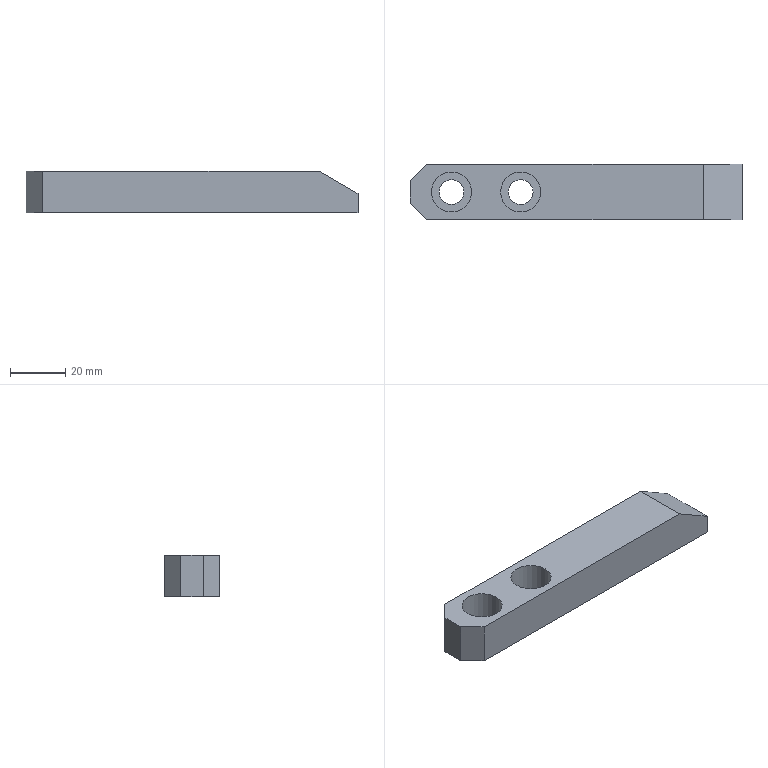Part | STEP file | lll_id830_x_t | 1 solid | 15 faces | box 120 x 20 x 15 mm | volume 30182 mm3 | plane 11 | cylinder 4 | commonest cylinder face diameters 9.009 x2 14.508 x2
STEP:
#1=CARTESIAN_POINT('',(3719.989,-179.337,0.));
#2=VERTEX_POINT('',#1);
#3=CARTESIAN_POINT('',(3727.243,-179.337,0.));
#4=DIRECTION('',(0.,0.,1.));
#5=DIRECTION('',(-1.,0.,0.));
#6=AXIS2_PLACEMENT_3D('',#3,#4,#5);
#7=CIRCLE('',#6,7.254);
#8=EDGE_CURVE('',#2,#2,#7,.T.);
#9=ORIENTED_EDGE('',*,*,#8,.F.);
#10=EDGE_LOOP('',(#9));
#11=FACE_BOUND('',#10,.T.);
#12=CARTESIAN_POINT('',(3694.989,-179.337,0.));
#13=VERTEX_POINT('',#12);
#14=CARTESIAN_POINT('',(3702.243,-179.337,0.));
#15=DIRECTION('',(0.,0.,1.));
#16=DIRECTION('',(-1.,0.,0.));
#17=AXIS2_PLACEMENT_3D('',#14,#15,#16);
#18=CIRCLE('',#17,7.254);
#19=EDGE_CURVE('',#13,#13,#18,.T.);
#20=ORIENTED_EDGE('',*,*,#19,.F.);
#21=EDGE_LOOP('',(#20));
#22=FACE_BOUND('',#21,.T.);
#23=CARTESIAN_POINT('',(3793.243,-169.337,0.));
#24=VERTEX_POINT('',#23);
#25=CARTESIAN_POINT('',(3693.243,-169.337,0.));
#26=VERTEX_POINT('',#25);
#27=CARTESIAN_POINT('',(3807.243,-169.337,0.));
#28=DIRECTION('',(-1.,0.,0.));
#29=VECTOR('',#28,1.);
#30=LINE('',#27,#29);
#31=EDGE_CURVE('',#24,#26,#30,.T.);
#32=ORIENTED_EDGE('',*,*,#31,.T.);
#33=CARTESIAN_POINT('',(3687.243,-175.337,0.));
#34=VERTEX_POINT('',#33);
#35=CARTESIAN_POINT('',(3687.243,-175.337,0.));
#36=DIRECTION('',(0.7071,0.7071,0.));
#37=VECTOR('',#36,1.);
#38=LINE('',#35,#37);
#39=EDGE_CURVE('',#34,#26,#38,.T.);
#40=ORIENTED_EDGE('',*,*,#39,.F.);
#41=CARTESIAN_POINT('',(3687.243,-183.337,0.));
#42=VERTEX_POINT('',#41);
#43=CARTESIAN_POINT('',(3687.243,-189.337,0.));
#44=DIRECTION('',(0.,1.,0.));
#45=VECTOR('',#44,1.);
#46=LINE('',#43,#45);
#47=EDGE_CURVE('',#42,#34,#46,.T.);
#48=ORIENTED_EDGE('',*,*,#47,.F.);
#49=CARTESIAN_POINT('',(3693.243,-189.337,0.));
#50=VERTEX_POINT('',#49);
#51=CARTESIAN_POINT('',(3693.243,-189.337,0.));
#52=DIRECTION('',(-0.7071,0.7071,0.));
#53=VECTOR('',#52,1.);
#54=LINE('',#51,#53);
#55=EDGE_CURVE('',#50,#42,#54,.T.);
#56=ORIENTED_EDGE('',*,*,#55,.F.);
#57=CARTESIAN_POINT('',(3793.243,-189.337,0.));
#58=VERTEX_POINT('',#57);
#59=CARTESIAN_POINT('',(3807.243,-189.337,0.));
#60=DIRECTION('',(-1.,0.,0.));
#61=VECTOR('',#60,1.);
#62=LINE('',#59,#61);
#63=EDGE_CURVE('',#58,#50,#62,.T.);
#64=ORIENTED_EDGE('',*,*,#63,.F.);
#65=CARTESIAN_POINT('',(3793.243,10.,0.));
#66=DIRECTION('',(0.,-1.,0.));
#67=VECTOR('',#66,1.);
#68=LINE('',#65,#67);
#69=EDGE_CURVE('',#24,#58,#68,.T.);
#70=ORIENTED_EDGE('',*,*,#69,.F.);
#71=EDGE_LOOP('',(#32,#40,#48,#56,#64,#70));
#72=FACE_BOUND('',#71,.T.);
#73=CARTESIAN_POINT('',(3807.243,-189.337,0.));
#74=DIRECTION('',(0.,0.,-1.));
#75=DIRECTION('',(1.,0.,0.));
#76=AXIS2_PLACEMENT_3D('',#73,#74,#75);
#77=PLANE('',#76);
#78=ADVANCED_FACE('',(#11,#22,#72),#77,.F.);
#79=CARTESIAN_POINT('',(3807.243,-169.337,-15.));
#80=VERTEX_POINT('',#79);
#81=CARTESIAN_POINT('',(3807.243,-169.337,-8.083));
#82=VERTEX_POINT('',#81);
#83=CARTESIAN_POINT('',(3807.243,-169.337,0.));
#84=DIRECTION('',(0.,0.,1.));
#85=VECTOR('',#84,1.);
#86=LINE('',#83,#85);
#87=EDGE_CURVE('',#80,#82,#86,.T.);
#88=ORIENTED_EDGE('',*,*,#87,.F.);
#89=CARTESIAN_POINT('',(3693.243,-169.337,-15.));
#90=VERTEX_POINT('',#89);
#91=CARTESIAN_POINT('',(3757.243,-169.337,-15.));
#92=DIRECTION('',(1.,0.,0.));
#93=VECTOR('',#92,1.);
#94=LINE('',#91,#93);
#95=EDGE_CURVE('',#90,#80,#94,.T.);
#96=ORIENTED_EDGE('',*,*,#95,.F.);
#97=CARTESIAN_POINT('',(3693.243,-169.337,-17.5));
#98=DIRECTION('',(0.,0.,-1.));
#99=VECTOR('',#98,1.);
#100=LINE('',#97,#99);
#101=EDGE_CURVE('',#26,#90,#100,.T.);
#102=ORIENTED_EDGE('',*,*,#101,.F.);
#103=ORIENTED_EDGE('',*,*,#31,.F.);
#104=CARTESIAN_POINT('',(3806.743,-169.337,-7.794));
#105=DIRECTION('',(-0.866,0.,0.5));
#106=VECTOR('',#105,1.);
#107=LINE('',#104,#106);
#108=EDGE_CURVE('',#82,#24,#107,.T.);
#109=ORIENTED_EDGE('',*,*,#108,.F.);
#110=EDGE_LOOP('',(#88,#96,#102,#103,#109));
#111=FACE_OUTER_BOUND('',#110,.T.);
#112=CARTESIAN_POINT('',(3757.243,-169.337,-17.5));
#113=DIRECTION('',(0.,-1.,0.));
#114=DIRECTION('',(0.,0.,-1.));
#115=AXIS2_PLACEMENT_3D('',#112,#113,#114);
#116=PLANE('',#115);
#117=ADVANCED_FACE('',(#111),#116,.F.);
#118=CARTESIAN_POINT('',(3687.243,-175.337,-15.));
#119=VERTEX_POINT('',#118);
#120=CARTESIAN_POINT('',(3687.243,-183.337,-15.));
#121=VERTEX_POINT('',#120);
#122=CARTESIAN_POINT('',(3687.243,10.,-15.));
#123=DIRECTION('',(0.,-1.,0.));
#124=VECTOR('',#123,1.);
#125=LINE('',#122,#124);
#126=EDGE_CURVE('',#119,#121,#125,.T.);
#127=ORIENTED_EDGE('',*,*,#126,.T.);
#128=CARTESIAN_POINT('',(3687.243,-183.337,0.));
#129=DIRECTION('',(0.,0.,-1.));
#130=VECTOR('',#129,1.);
#131=LINE('',#128,#130);
#132=EDGE_CURVE('',#42,#121,#131,.T.);
#133=ORIENTED_EDGE('',*,*,#132,.F.);
#134=ORIENTED_EDGE('',*,*,#47,.T.);
#135=CARTESIAN_POINT('',(3687.243,-175.337,0.));
#136=DIRECTION('',(0.,0.,1.));
#137=VECTOR('',#136,1.);
#138=LINE('',#135,#137);
#139=EDGE_CURVE('',#119,#34,#138,.T.);
#140=ORIENTED_EDGE('',*,*,#139,.F.);
#141=EDGE_LOOP('',(#127,#133,#134,#140));
#142=FACE_OUTER_BOUND('',#141,.T.);
#143=CARTESIAN_POINT('',(3687.243,10.,0.));
#144=DIRECTION('',(1.,0.,0.));
#145=DIRECTION('',(0.,0.,1.));
#146=AXIS2_PLACEMENT_3D('',#143,#144,#145);
#147=PLANE('',#146);
#148=ADVANCED_FACE('',(#142),#147,.F.);
#149=CARTESIAN_POINT('',(3807.243,-189.337,-15.));
#150=VERTEX_POINT('',#149);
#151=CARTESIAN_POINT('',(3807.243,-189.337,-8.083));
#152=VERTEX_POINT('',#151);
#153=CARTESIAN_POINT('',(3807.243,-189.337,-35.));
#154=DIRECTION('',(0.,0.,1.));
#155=VECTOR('',#154,1.);
#156=LINE('',#153,#155);
#157=EDGE_CURVE('',#150,#152,#156,.T.);
#158=ORIENTED_EDGE('',*,*,#157,.F.);
#159=CARTESIAN_POINT('',(3807.243,10.,-15.));
#160=DIRECTION('',(0.,1.,0.));
#161=VECTOR('',#160,1.);
#162=LINE('',#159,#161);
#163=EDGE_CURVE('',#150,#80,#162,.T.);
#164=ORIENTED_EDGE('',*,*,#163,.T.);
#165=ORIENTED_EDGE('',*,*,#87,.T.);
#166=CARTESIAN_POINT('',(3807.243,10.,-8.083));
#167=DIRECTION('',(0.,1.,0.));
#168=VECTOR('',#167,1.);
#169=LINE('',#166,#168);
#170=EDGE_CURVE('',#152,#82,#169,.T.);
#171=ORIENTED_EDGE('',*,*,#170,.F.);
#172=EDGE_LOOP('',(#158,#164,#165,#171));
#173=FACE_OUTER_BOUND('',#172,.T.);
#174=CARTESIAN_POINT('',(3807.243,10.,0.));
#175=DIRECTION('',(1.,0.,0.));
#176=DIRECTION('',(0.,0.,1.));
#177=AXIS2_PLACEMENT_3D('',#174,#175,#176);
#178=PLANE('',#177);
#179=ADVANCED_FACE('',(#173),#178,.T.);
#180=ORIENTED_EDGE('',*,*,#63,.T.);
#181=CARTESIAN_POINT('',(3693.243,-189.337,-15.));
#182=VERTEX_POINT('',#181);
#183=CARTESIAN_POINT('',(3693.243,-189.337,-35.));
#184=DIRECTION('',(0.,0.,1.));
#185=VECTOR('',#184,1.);
#186=LINE('',#183,#185);
#187=EDGE_CURVE('',#182,#50,#186,.T.);
#188=ORIENTED_EDGE('',*,*,#187,.F.);
#189=CARTESIAN_POINT('',(3807.243,-189.337,-15.));
#190=DIRECTION('',(1.,0.,0.));
#191=VECTOR('',#190,1.);
#192=LINE('',#189,#191);
#193=EDGE_CURVE('',#182,#150,#192,.T.);
#194=ORIENTED_EDGE('',*,*,#193,.T.);
#195=ORIENTED_EDGE('',*,*,#157,.T.);
#196=CARTESIAN_POINT('',(3806.743,-189.337,-7.794));
#197=DIRECTION('',(0.866,0.,-0.5));
#198=VECTOR('',#197,1.);
#199=LINE('',#196,#198);
#200=EDGE_CURVE('',#58,#152,#199,.T.);
#201=ORIENTED_EDGE('',*,*,#200,.F.);
#202=EDGE_LOOP('',(#180,#188,#194,#195,#201));
#203=FACE_OUTER_BOUND('',#202,.T.);
#204=CARTESIAN_POINT('',(3807.243,-189.337,-35.));
#205=DIRECTION('',(0.,1.,0.));
#206=DIRECTION('',(0.,0.,1.));
#207=AXIS2_PLACEMENT_3D('',#204,#205,#206);
#208=PLANE('',#207);
#209=ADVANCED_FACE('',(#203),#208,.F.);
#210=CARTESIAN_POINT('',(3722.739,-179.337,-15.));
#211=VERTEX_POINT('',#210);
#212=CARTESIAN_POINT('',(3727.243,-179.337,-15.));
#213=DIRECTION('',(0.,0.,-1.));
#214=DIRECTION('',(-1.,0.,0.));
#215=AXIS2_PLACEMENT_3D('',#212,#213,#214);
#216=CIRCLE('',#215,4.505);
#217=EDGE_CURVE('',#211,#211,#216,.T.);
#218=ORIENTED_EDGE('',*,*,#217,.F.);
#219=EDGE_LOOP('',(#218));
#220=FACE_BOUND('',#219,.T.);
#221=CARTESIAN_POINT('',(3697.739,-179.337,-15.));
#222=VERTEX_POINT('',#221);
#223=CARTESIAN_POINT('',(3702.243,-179.337,-15.));
#224=DIRECTION('',(0.,0.,-1.));
#225=DIRECTION('',(-1.,0.,0.));
#226=AXIS2_PLACEMENT_3D('',#223,#224,#225);
#227=CIRCLE('',#226,4.505);
#228=EDGE_CURVE('',#222,#222,#227,.T.);
#229=ORIENTED_EDGE('',*,*,#228,.F.);
#230=EDGE_LOOP('',(#229));
#231=FACE_BOUND('',#230,.T.);
#232=ORIENTED_EDGE('',*,*,#95,.T.);
#233=ORIENTED_EDGE('',*,*,#163,.F.);
#234=ORIENTED_EDGE('',*,*,#193,.F.);
#235=CARTESIAN_POINT('',(3693.243,-189.337,-15.));
#236=DIRECTION('',(0.7071,-0.7071,0.));
#237=VECTOR('',#236,1.);
#238=LINE('',#235,#237);
#239=EDGE_CURVE('',#121,#182,#238,.T.);
#240=ORIENTED_EDGE('',*,*,#239,.F.);
#241=ORIENTED_EDGE('',*,*,#126,.F.);
#242=CARTESIAN_POINT('',(3687.243,-175.337,-15.));
#243=DIRECTION('',(-0.7071,-0.7071,0.));
#244=VECTOR('',#243,1.);
#245=LINE('',#242,#244);
#246=EDGE_CURVE('',#90,#119,#245,.T.);
#247=ORIENTED_EDGE('',*,*,#246,.F.);
#248=EDGE_LOOP('',(#232,#233,#234,#240,#241,#247));
#249=FACE_BOUND('',#248,.T.);
#250=CARTESIAN_POINT('',(3757.243,-179.337,-15.));
#251=DIRECTION('',(0.,0.,1.));
#252=DIRECTION('',(-1.,0.,0.));
#253=AXIS2_PLACEMENT_3D('',#250,#251,#252);
#254=PLANE('',#253);
#255=ADVANCED_FACE('',(#220,#231,#249),#254,.F.);
#256=CARTESIAN_POINT('',(3697.739,-179.337,-11.));
#257=VERTEX_POINT('',#256);
#258=CARTESIAN_POINT('',(3702.243,-179.337,-11.));
#259=DIRECTION('',(0.,0.,1.));
#260=DIRECTION('',(-1.,0.,0.));
#261=AXIS2_PLACEMENT_3D('',#258,#259,#260);
#262=CIRCLE('',#261,4.505);
#263=EDGE_CURVE('',#257,#257,#262,.T.);
#264=ORIENTED_EDGE('',*,*,#263,.T.);
#265=EDGE_LOOP('',(#264));
#266=FACE_BOUND('',#265,.T.);
#267=ORIENTED_EDGE('',*,*,#228,.T.);
#268=EDGE_LOOP('',(#267));
#269=FACE_BOUND('',#268,.T.);
#270=CARTESIAN_POINT('',(3702.243,-179.337,0.));
#271=DIRECTION('',(0.,0.,-1.));
#272=DIRECTION('',(1.,0.,0.));
#273=AXIS2_PLACEMENT_3D('',#270,#271,#272);
#274=CYLINDRICAL_SURFACE('',#273,4.505);
#275=ADVANCED_FACE('',(#266,#269),#274,.F.);
#276=ORIENTED_EDGE('',*,*,#263,.F.);
#277=EDGE_LOOP('',(#276));
#278=FACE_BOUND('',#277,.T.);
#279=CARTESIAN_POINT('',(3694.989,-179.337,-11.));
#280=VERTEX_POINT('',#279);
#281=CARTESIAN_POINT('',(3702.243,-179.337,-11.));
#282=DIRECTION('',(0.,0.,1.));
#283=DIRECTION('',(-1.,0.,0.));
#284=AXIS2_PLACEMENT_3D('',#281,#282,#283);
#285=CIRCLE('',#284,7.254);
#286=EDGE_CURVE('',#280,#280,#285,.T.);
#287=ORIENTED_EDGE('',*,*,#286,.T.);
#288=EDGE_LOOP('',(#287));
#289=FACE_BOUND('',#288,.T.);
#290=CARTESIAN_POINT('',(3702.243,-179.337,-11.));
#291=DIRECTION('',(0.,0.,-1.));
#292=DIRECTION('',(1.,0.,0.));
#293=AXIS2_PLACEMENT_3D('',#290,#291,#292);
#294=PLANE('',#293);
#295=ADVANCED_FACE('',(#278,#289),#294,.F.);
#296=ORIENTED_EDGE('',*,*,#286,.F.);
#297=EDGE_LOOP('',(#296));
#298=FACE_BOUND('',#297,.T.);
#299=ORIENTED_EDGE('',*,*,#19,.T.);
#300=EDGE_LOOP('',(#299));
#301=FACE_BOUND('',#300,.T.);
#302=CARTESIAN_POINT('',(3702.243,-179.337,0.));
#303=DIRECTION('',(0.,0.,-1.));
#304=DIRECTION('',(1.,0.,0.));
#305=AXIS2_PLACEMENT_3D('',#302,#303,#304);
#306=CYLINDRICAL_SURFACE('',#305,7.254);
#307=ADVANCED_FACE('',(#298,#301),#306,.F.);
#308=CARTESIAN_POINT('',(3722.739,-179.337,-11.));
#309=VERTEX_POINT('',#308);
#310=CARTESIAN_POINT('',(3727.243,-179.337,-11.));
#311=DIRECTION('',(0.,0.,1.));
#312=DIRECTION('',(-1.,0.,0.));
#313=AXIS2_PLACEMENT_3D('',#310,#311,#312);
#314=CIRCLE('',#313,4.505);
#315=EDGE_CURVE('',#309,#309,#314,.T.);
#316=ORIENTED_EDGE('',*,*,#315,.T.);
#317=EDGE_LOOP('',(#316));
#318=FACE_BOUND('',#317,.T.);
#319=ORIENTED_EDGE('',*,*,#217,.T.);
#320=EDGE_LOOP('',(#319));
#321=FACE_BOUND('',#320,.T.);
#322=CARTESIAN_POINT('',(3727.243,-179.337,0.));
#323=DIRECTION('',(0.,0.,-1.));
#324=DIRECTION('',(1.,0.,0.));
#325=AXIS2_PLACEMENT_3D('',#322,#323,#324);
#326=CYLINDRICAL_SURFACE('',#325,4.505);
#327=ADVANCED_FACE('',(#318,#321),#326,.F.);
#328=ORIENTED_EDGE('',*,*,#315,.F.);
#329=EDGE_LOOP('',(#328));
#330=FACE_BOUND('',#329,.T.);
#331=CARTESIAN_POINT('',(3719.989,-179.337,-11.));
#332=VERTEX_POINT('',#331);
#333=CARTESIAN_POINT('',(3727.243,-179.337,-11.));
#334=DIRECTION('',(0.,0.,1.));
#335=DIRECTION('',(-1.,0.,0.));
#336=AXIS2_PLACEMENT_3D('',#333,#334,#335);
#337=CIRCLE('',#336,7.254);
#338=EDGE_CURVE('',#332,#332,#337,.T.);
#339=ORIENTED_EDGE('',*,*,#338,.T.);
#340=EDGE_LOOP('',(#339));
#341=FACE_BOUND('',#340,.T.);
#342=CARTESIAN_POINT('',(3727.243,-179.337,-11.));
#343=DIRECTION('',(0.,0.,-1.));
#344=DIRECTION('',(1.,0.,0.));
#345=AXIS2_PLACEMENT_3D('',#342,#343,#344);
#346=PLANE('',#345);
#347=ADVANCED_FACE('',(#330,#341),#346,.F.);
#348=ORIENTED_EDGE('',*,*,#338,.F.);
#349=EDGE_LOOP('',(#348));
#350=FACE_BOUND('',#349,.T.);
#351=ORIENTED_EDGE('',*,*,#8,.T.);
#352=EDGE_LOOP('',(#351));
#353=FACE_BOUND('',#352,.T.);
#354=CARTESIAN_POINT('',(3727.243,-179.337,0.));
#355=DIRECTION('',(0.,0.,-1.));
#356=DIRECTION('',(1.,0.,0.));
#357=AXIS2_PLACEMENT_3D('',#354,#355,#356);
#358=CYLINDRICAL_SURFACE('',#357,7.254);
#359=ADVANCED_FACE('',(#350,#353),#358,.F.);
#360=ORIENTED_EDGE('',*,*,#246,.T.);
#361=ORIENTED_EDGE('',*,*,#139,.T.);
#362=ORIENTED_EDGE('',*,*,#39,.T.);
#363=ORIENTED_EDGE('',*,*,#101,.T.);
#364=EDGE_LOOP('',(#360,#361,#362,#363));
#365=FACE_OUTER_BOUND('',#364,.T.);
#366=CARTESIAN_POINT('',(3687.243,-175.337,0.));
#367=DIRECTION('',(0.7071,-0.7071,0.));
#368=DIRECTION('',(0.,0.,-1.));
#369=AXIS2_PLACEMENT_3D('',#366,#367,#368);
#370=PLANE('',#369);
#371=ADVANCED_FACE('',(#365),#370,.F.);
#372=ORIENTED_EDGE('',*,*,#239,.T.);
#373=ORIENTED_EDGE('',*,*,#187,.T.);
#374=ORIENTED_EDGE('',*,*,#55,.T.);
#375=ORIENTED_EDGE('',*,*,#132,.T.);
#376=EDGE_LOOP('',(#372,#373,#374,#375));
#377=FACE_OUTER_BOUND('',#376,.T.);
#378=CARTESIAN_POINT('',(3693.243,-189.337,-35.));
#379=DIRECTION('',(0.7071,0.7071,0.));
#380=DIRECTION('',(0.,0.,-1.));
#381=AXIS2_PLACEMENT_3D('',#378,#379,#380);
#382=PLANE('',#381);
#383=ADVANCED_FACE('',(#377),#382,.F.);
#384=ORIENTED_EDGE('',*,*,#200,.T.);
#385=ORIENTED_EDGE('',*,*,#170,.T.);
#386=ORIENTED_EDGE('',*,*,#108,.T.);
#387=ORIENTED_EDGE('',*,*,#69,.T.);
#388=EDGE_LOOP('',(#384,#385,#386,#387));
#389=FACE_OUTER_BOUND('',#388,.T.);
#390=CARTESIAN_POINT('',(3806.743,10.,-7.794));
#391=DIRECTION('',(0.5,0.,0.866));
#392=DIRECTION('',(0.,1.,0.));
#393=AXIS2_PLACEMENT_3D('',#390,#391,#392);
#394=PLANE('',#393);
#395=ADVANCED_FACE('',(#389),#394,.T.);
#396=CLOSED_SHELL('',(#78,#117,#148,#179,#209,#255,#275,#295,#307,#327,#347,#359,#371,#383,#395));
#397=MANIFOLD_SOLID_BREP('',#396);
#398=(LENGTH_UNIT()NAMED_UNIT(*)SI_UNIT(.MILLI.,.METRE.));
#399=UNCERTAINTY_MEASURE_WITH_UNIT(LENGTH_MEASURE(0.00002),#398,'','');
#400=(NAMED_UNIT(*)PLANE_ANGLE_UNIT()SI_UNIT($,.RADIAN.));
#401=PLANE_ANGLE_MEASURE_WITH_UNIT(PLANE_ANGLE_MEASURE(0.01745),#400);
#402=DIMENSIONAL_EXPONENTS(0.,0.,0.,0.,0.,0.,0.);
#403=(CONVERSION_BASED_UNIT('DEGREE',#401)NAMED_UNIT(#402)PLANE_ANGLE_UNIT());
#404=(NAMED_UNIT(*)SI_UNIT($,.STERADIAN.)SOLID_ANGLE_UNIT());
#405=(GEOMETRIC_REPRESENTATION_CONTEXT(3)GLOBAL_UNCERTAINTY_ASSIGNED_CONTEXT((#399))GLOBAL_UNIT_ASSIGNED_CONTEXT((#398,#403,#404))REPRESENTATION_CONTEXT('',''));
#406=ADVANCED_BREP_SHAPE_REPRESENTATION('',(#397),#405);